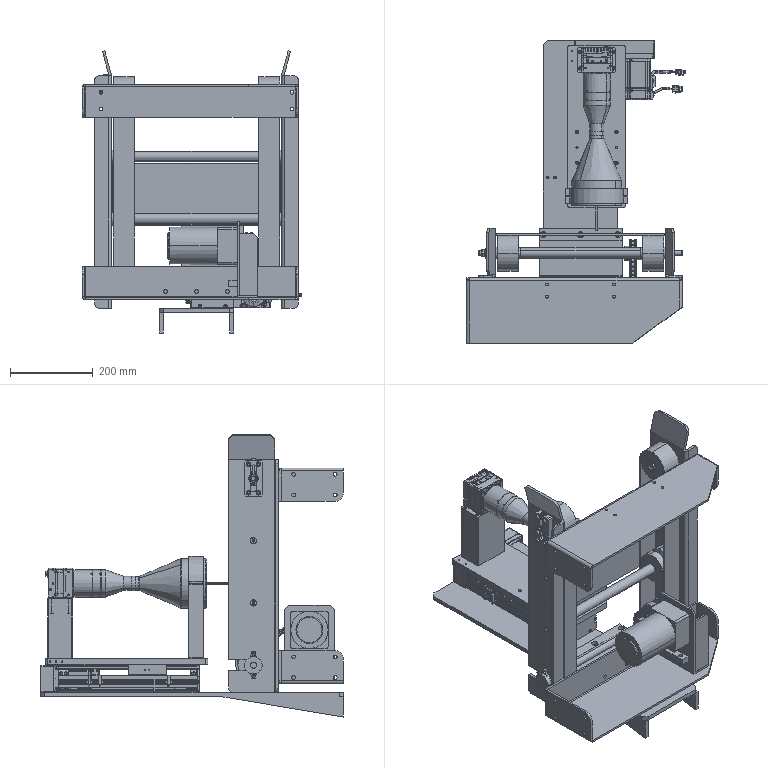Part | SolidWorks | 155 solids | 7084 faces | volume 13967831 mm3 | plane 3094 | cylinder 2947 | cone 513 | sphere 256 | torus 200 | spline 74 | commonest cylinder face diameters 4.45 x288 11.81 x216 57.066 x144 2 x120 5 x108 3.3 x100